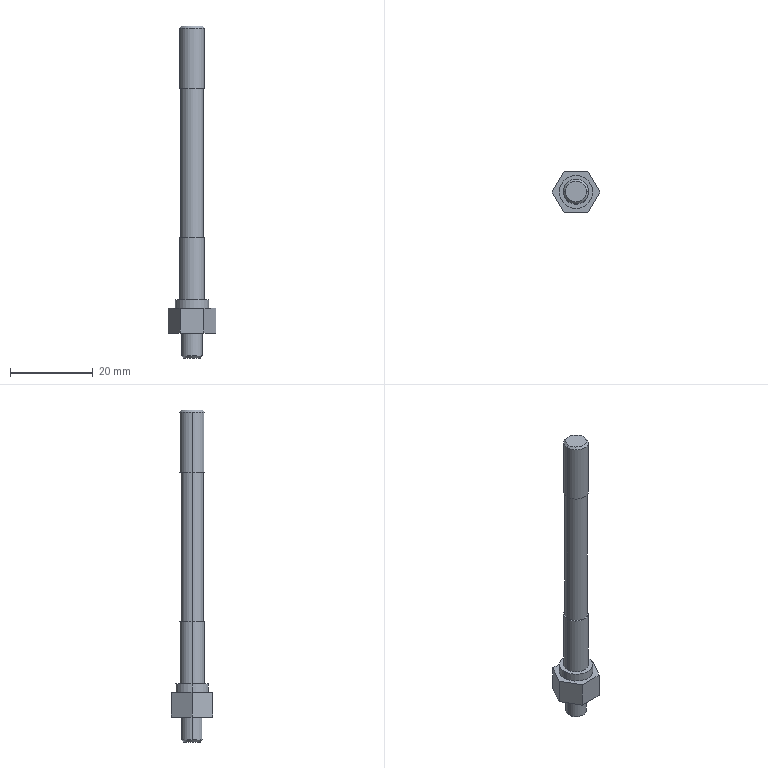Part | SolidWorks | features ICE 3, Chamfer 2, Extrusion 1, RefAxis 1, RevCut 1 | 1 solid | 27 faces | box 11.547 x 10 x 80 mm | volume 2437 mm3 | plane 13 | cylinder 10 | cone 4 | commonest cylinder face diameters 6 x4 5 x2 5.5 x2 8 x2
STEP:
#1=CARTESIAN_POINT('',(-2.,0.,-6.));
#2=VERTEX_POINT('',#1);
#3=CARTESIAN_POINT('',(2.,0.,-6.));
#4=VERTEX_POINT('',#3);
#5=CARTESIAN_POINT('',(0.,0.,-6.));
#6=DIRECTION('',(0.,0.,-1.));
#7=DIRECTION('',(-1.,0.,0.));
#8=AXIS2_PLACEMENT_3D('',#5,#6,#7);
#9=CIRCLE('',#8,2.);
#10=EDGE_CURVE('',#2,#4,#9,.T.);
#11=ORIENTED_EDGE('',*,*,#10,.F.);
#12=CARTESIAN_POINT('',(-2.5,0.,-5.5));
#13=VERTEX_POINT('',#12);
#14=CARTESIAN_POINT('',(-2.,0.,-6.));
#15=DIRECTION('',(-0.7071,0.,0.7071));
#16=VECTOR('',#15,1000.);
#17=LINE('',#14,#16);
#18=EDGE_CURVE('',#2,#13,#17,.T.);
#19=ORIENTED_EDGE('',*,*,#18,.T.);
#20=CARTESIAN_POINT('',(2.5,0.,-5.5));
#21=VERTEX_POINT('',#20);
#22=CARTESIAN_POINT('',(0.,0.,-5.5));
#23=DIRECTION('',(0.,0.,1.));
#24=DIRECTION('',(-1.,0.,0.));
#25=AXIS2_PLACEMENT_3D('',#22,#23,#24);
#26=CIRCLE('',#25,2.5);
#27=EDGE_CURVE('',#21,#13,#26,.T.);
#28=ORIENTED_EDGE('',*,*,#27,.F.);
#29=CARTESIAN_POINT('',(2.,0.,-6.));
#30=DIRECTION('',(0.7071,0.,0.7071));
#31=VECTOR('',#30,1000.);
#32=LINE('',#29,#31);
#33=EDGE_CURVE('',#4,#21,#32,.T.);
#34=ORIENTED_EDGE('',*,*,#33,.F.);
#35=EDGE_LOOP('',(#11,#19,#28,#34));
#36=FACE_OUTER_BOUND('',#35,.T.);
#37=CARTESIAN_POINT('',(0.,0.,-6.));
#38=DIRECTION('',(0.,0.,1.));
#39=DIRECTION('',(1.,0.,0.));
#40=AXIS2_PLACEMENT_3D('',#37,#38,#39);
#41=CONICAL_SURFACE('',#40,2.,0.7854);
#42=ADVANCED_FACE('',(#36),#41,.T.);
#43=CARTESIAN_POINT('',(-3.,0.,73.5));
#44=VERTEX_POINT('',#43);
#45=CARTESIAN_POINT('',(3.,0.,73.5));
#46=VERTEX_POINT('',#45);
#47=CARTESIAN_POINT('',(0.,0.,73.5));
#48=DIRECTION('',(0.,0.,-1.));
#49=DIRECTION('',(1.,0.,0.));
#50=AXIS2_PLACEMENT_3D('',#47,#48,#49);
#51=CIRCLE('',#50,3.);
#52=EDGE_CURVE('',#44,#46,#51,.T.);
#53=ORIENTED_EDGE('',*,*,#52,.T.);
#54=CARTESIAN_POINT('',(3.,0.,59.));
#55=VERTEX_POINT('',#54);
#56=CARTESIAN_POINT('',(3.,0.,74.));
#57=DIRECTION('',(0.,0.,-1.));
#58=VECTOR('',#57,1000.);
#59=LINE('',#56,#58);
#60=EDGE_CURVE('',#46,#55,#59,.T.);
#61=ORIENTED_EDGE('',*,*,#60,.T.);
#62=CARTESIAN_POINT('',(-3.,0.,59.));
#63=VERTEX_POINT('',#62);
#64=CARTESIAN_POINT('',(0.,0.,59.));
#65=DIRECTION('',(0.,0.,1.));
#66=DIRECTION('',(1.,0.,0.));
#67=AXIS2_PLACEMENT_3D('',#64,#65,#66);
#68=CIRCLE('',#67,3.);
#69=EDGE_CURVE('',#55,#63,#68,.T.);
#70=ORIENTED_EDGE('',*,*,#69,.T.);
#71=CARTESIAN_POINT('',(-3.,0.,74.));
#72=DIRECTION('',(0.,0.,-1.));
#73=VECTOR('',#72,1000.);
#74=LINE('',#71,#73);
#75=EDGE_CURVE('',#44,#63,#74,.T.);
#76=ORIENTED_EDGE('',*,*,#75,.F.);
#77=EDGE_LOOP('',(#53,#61,#70,#76));
#78=FACE_OUTER_BOUND('',#77,.T.);
#79=CARTESIAN_POINT('',(0.,0.,74.));
#80=DIRECTION('',(0.,0.,-1.));
#81=DIRECTION('',(-1.,0.,0.));
#82=AXIS2_PLACEMENT_3D('',#79,#80,#81);
#83=CYLINDRICAL_SURFACE('',#82,3.);
#84=ADVANCED_FACE('',(#78),#83,.T.);
#85=CARTESIAN_POINT('',(2.5,0.,74.));
#86=VERTEX_POINT('',#85);
#87=CARTESIAN_POINT('',(-2.5,0.,74.));
#88=VERTEX_POINT('',#87);
#89=CARTESIAN_POINT('',(0.,0.,74.));
#90=DIRECTION('',(0.,0.,1.));
#91=DIRECTION('',(1.,0.,0.));
#92=AXIS2_PLACEMENT_3D('',#89,#90,#91);
#93=CIRCLE('',#92,2.5);
#94=EDGE_CURVE('',#86,#88,#93,.T.);
#95=ORIENTED_EDGE('',*,*,#94,.F.);
#96=CARTESIAN_POINT('',(2.5,0.,74.));
#97=DIRECTION('',(0.7071,0.,-0.7071));
#98=VECTOR('',#97,1000.);
#99=LINE('',#96,#98);
#100=EDGE_CURVE('',#86,#46,#99,.T.);
#101=ORIENTED_EDGE('',*,*,#100,.T.);
#102=ORIENTED_EDGE('',*,*,#52,.F.);
#103=CARTESIAN_POINT('',(-2.5,0.,74.));
#104=DIRECTION('',(-0.7071,0.,-0.7071));
#105=VECTOR('',#104,1000.);
#106=LINE('',#103,#105);
#107=EDGE_CURVE('',#88,#44,#106,.T.);
#108=ORIENTED_EDGE('',*,*,#107,.F.);
#109=EDGE_LOOP('',(#95,#101,#102,#108));
#110=FACE_OUTER_BOUND('',#109,.T.);
#111=CARTESIAN_POINT('',(0.,0.,74.));
#112=DIRECTION('',(0.,0.,-1.));
#113=DIRECTION('',(-1.,0.,0.));
#114=AXIS2_PLACEMENT_3D('',#111,#112,#113);
#115=CONICAL_SURFACE('',#114,2.5,0.7854);
#116=ADVANCED_FACE('',(#110),#115,.T.);
#117=CARTESIAN_POINT('',(2.75,0.,23.));
#118=VERTEX_POINT('',#117);
#119=CARTESIAN_POINT('',(-2.75,0.,23.));
#120=VERTEX_POINT('',#119);
#121=CARTESIAN_POINT('',(0.,0.,23.));
#122=DIRECTION('',(0.,0.,1.));
#123=DIRECTION('',(1.,0.,0.));
#124=AXIS2_PLACEMENT_3D('',#121,#122,#123);
#125=CIRCLE('',#124,2.75);
#126=EDGE_CURVE('',#118,#120,#125,.T.);
#127=ORIENTED_EDGE('',*,*,#126,.T.);
#128=CARTESIAN_POINT('',(-2.75,0.,59.));
#129=VERTEX_POINT('',#128);
#130=CARTESIAN_POINT('',(-2.75,0.,73.5));
#131=DIRECTION('',(0.,0.,1.));
#132=VECTOR('',#131,1000.);
#133=LINE('',#130,#132);
#134=EDGE_CURVE('',#120,#129,#133,.T.);
#135=ORIENTED_EDGE('',*,*,#134,.T.);
#136=CARTESIAN_POINT('',(2.75,0.,59.));
#137=VERTEX_POINT('',#136);
#138=CARTESIAN_POINT('',(0.,0.,59.));
#139=DIRECTION('',(0.,0.,1.));
#140=DIRECTION('',(1.,0.,0.));
#141=AXIS2_PLACEMENT_3D('',#138,#139,#140);
#142=CIRCLE('',#141,2.75);
#143=EDGE_CURVE('',#137,#129,#142,.T.);
#144=ORIENTED_EDGE('',*,*,#143,.F.);
#145=CARTESIAN_POINT('',(2.75,0.,73.5));
#146=DIRECTION('',(0.,0.,1.));
#147=VECTOR('',#146,1000.);
#148=LINE('',#145,#147);
#149=EDGE_CURVE('',#118,#137,#148,.T.);
#150=ORIENTED_EDGE('',*,*,#149,.F.);
#151=EDGE_LOOP('',(#127,#135,#144,#150));
#152=FACE_OUTER_BOUND('',#151,.T.);
#153=CARTESIAN_POINT('',(0.,0.,73.5));
#154=DIRECTION('',(0.,0.,1.));
#155=DIRECTION('',(1.,0.,0.));
#156=AXIS2_PLACEMENT_3D('',#153,#154,#155);
#157=CYLINDRICAL_SURFACE('',#156,2.75);
#158=ADVANCED_FACE('',(#152),#157,.T.);
#159=CARTESIAN_POINT('',(-3.,0.,23.));
#160=VERTEX_POINT('',#159);
#161=CARTESIAN_POINT('',(3.,0.,23.));
#162=VERTEX_POINT('',#161);
#163=CARTESIAN_POINT('',(0.,0.,23.));
#164=DIRECTION('',(0.,0.,-1.));
#165=DIRECTION('',(-1.,0.,0.));
#166=AXIS2_PLACEMENT_3D('',#163,#164,#165);
#167=CIRCLE('',#166,3.);
#168=EDGE_CURVE('',#160,#162,#167,.T.);
#169=ORIENTED_EDGE('',*,*,#168,.T.);
#170=CARTESIAN_POINT('',(3.,0.,8.));
#171=VERTEX_POINT('',#170);
#172=CARTESIAN_POINT('',(3.,0.,74.));
#173=DIRECTION('',(0.,0.,-1.));
#174=VECTOR('',#173,1000.);
#175=LINE('',#172,#174);
#176=EDGE_CURVE('',#162,#171,#175,.T.);
#177=ORIENTED_EDGE('',*,*,#176,.T.);
#178=CARTESIAN_POINT('',(-3.,0.,8.));
#179=VERTEX_POINT('',#178);
#180=CARTESIAN_POINT('',(0.,0.,8.));
#181=DIRECTION('',(0.,0.,1.));
#182=DIRECTION('',(1.,0.,0.));
#183=AXIS2_PLACEMENT_3D('',#180,#181,#182);
#184=CIRCLE('',#183,3.);
#185=EDGE_CURVE('',#171,#179,#184,.T.);
#186=ORIENTED_EDGE('',*,*,#185,.T.);
#187=CARTESIAN_POINT('',(-3.,0.,74.));
#188=DIRECTION('',(0.,0.,-1.));
#189=VECTOR('',#188,1000.);
#190=LINE('',#187,#189);
#191=EDGE_CURVE('',#160,#179,#190,.T.);
#192=ORIENTED_EDGE('',*,*,#191,.F.);
#193=EDGE_LOOP('',(#169,#177,#186,#192));
#194=FACE_OUTER_BOUND('',#193,.T.);
#195=CARTESIAN_POINT('',(0.,0.,74.));
#196=DIRECTION('',(0.,0.,-1.));
#197=DIRECTION('',(-1.,0.,0.));
#198=AXIS2_PLACEMENT_3D('',#195,#196,#197);
#199=CYLINDRICAL_SURFACE('',#198,3.);
#200=ADVANCED_FACE('',(#194),#199,.T.);
#201=CARTESIAN_POINT('',(4.,0.,8.));
#202=VERTEX_POINT('',#201);
#203=CARTESIAN_POINT('',(-4.,0.,8.));
#204=VERTEX_POINT('',#203);
#205=CARTESIAN_POINT('',(0.,0.,8.));
#206=DIRECTION('',(0.,0.,1.));
#207=DIRECTION('',(1.,0.,0.));
#208=AXIS2_PLACEMENT_3D('',#205,#206,#207);
#209=CIRCLE('',#208,4.);
#210=EDGE_CURVE('',#202,#204,#209,.T.);
#211=ORIENTED_EDGE('',*,*,#210,.F.);
#212=CARTESIAN_POINT('',(4.,0.,6.));
#213=VERTEX_POINT('',#212);
#214=CARTESIAN_POINT('',(4.,0.,8.));
#215=DIRECTION('',(0.,0.,-1.));
#216=VECTOR('',#215,1000.);
#217=LINE('',#214,#216);
#218=EDGE_CURVE('',#202,#213,#217,.T.);
#219=ORIENTED_EDGE('',*,*,#218,.T.);
#220=CARTESIAN_POINT('',(-4.,0.,6.));
#221=VERTEX_POINT('',#220);
#222=CARTESIAN_POINT('',(0.,0.,6.));
#223=DIRECTION('',(0.,0.,1.));
#224=DIRECTION('',(1.,0.,0.));
#225=AXIS2_PLACEMENT_3D('',#222,#223,#224);
#226=CIRCLE('',#225,4.);
#227=EDGE_CURVE('',#213,#221,#226,.T.);
#228=ORIENTED_EDGE('',*,*,#227,.T.);
#229=CARTESIAN_POINT('',(-4.,0.,8.));
#230=DIRECTION('',(0.,0.,-1.));
#231=VECTOR('',#230,1000.);
#232=LINE('',#229,#231);
#233=EDGE_CURVE('',#204,#221,#232,.T.);
#234=ORIENTED_EDGE('',*,*,#233,.F.);
#235=EDGE_LOOP('',(#211,#219,#228,#234));
#236=FACE_OUTER_BOUND('',#235,.T.);
#237=CARTESIAN_POINT('',(0.,0.,8.));
#238=DIRECTION('',(0.,0.,-1.));
#239=DIRECTION('',(-1.,0.,0.));
#240=AXIS2_PLACEMENT_3D('',#237,#238,#239);
#241=CYLINDRICAL_SURFACE('',#240,4.);
#242=ADVANCED_FACE('',(#236),#241,.T.);
#243=ORIENTED_EDGE('',*,*,#27,.T.);
#244=CARTESIAN_POINT('',(-2.5,0.,0.));
#245=VERTEX_POINT('',#244);
#246=CARTESIAN_POINT('',(-2.5,0.,-6.));
#247=DIRECTION('',(0.,0.,1.));
#248=VECTOR('',#247,1000.);
#249=LINE('',#246,#248);
#250=EDGE_CURVE('',#13,#245,#249,.T.);
#251=ORIENTED_EDGE('',*,*,#250,.T.);
#252=CARTESIAN_POINT('',(2.5,0.,0.));
#253=VERTEX_POINT('',#252);
#254=CARTESIAN_POINT('',(0.,0.,0.));
#255=DIRECTION('',(0.,0.,-1.));
#256=DIRECTION('',(1.,0.,0.));
#257=AXIS2_PLACEMENT_3D('',#254,#255,#256);
#258=CIRCLE('',#257,2.5);
#259=EDGE_CURVE('',#245,#253,#258,.T.);
#260=ORIENTED_EDGE('',*,*,#259,.T.);
#261=CARTESIAN_POINT('',(2.5,0.,-6.));
#262=DIRECTION('',(0.,0.,1.));
#263=VECTOR('',#262,1000.);
#264=LINE('',#261,#263);
#265=EDGE_CURVE('',#21,#253,#264,.T.);
#266=ORIENTED_EDGE('',*,*,#265,.F.);
#267=EDGE_LOOP('',(#243,#251,#260,#266));
#268=FACE_OUTER_BOUND('',#267,.T.);
#269=CARTESIAN_POINT('',(0.,0.,-6.));
#270=DIRECTION('',(0.,0.,1.));
#271=DIRECTION('',(1.,0.,0.));
#272=AXIS2_PLACEMENT_3D('',#269,#270,#271);
#273=CYLINDRICAL_SURFACE('',#272,2.5);
#274=ADVANCED_FACE('',(#268),#273,.T.);
#275=CARTESIAN_POINT('',(0.,0.,8.));
#276=DIRECTION('',(0.,0.,1.));
#277=DIRECTION('',(1.,0.,0.));
#278=AXIS2_PLACEMENT_3D('',#275,#276,#277);
#279=CIRCLE('',#278,4.);
#280=EDGE_CURVE('',#204,#202,#279,.T.);
#281=ORIENTED_EDGE('',*,*,#280,.T.);
#282=ORIENTED_EDGE('',*,*,#210,.T.);
#283=EDGE_LOOP('',(#281,#282));
#284=FACE_OUTER_BOUND('',#283,.T.);
#285=CARTESIAN_POINT('',(0.,0.,8.));
#286=DIRECTION('',(0.,0.,1.));
#287=DIRECTION('',(1.,0.,0.));
#288=AXIS2_PLACEMENT_3D('',#285,#286,#287);
#289=CIRCLE('',#288,3.);
#290=EDGE_CURVE('',#179,#171,#289,.T.);
#291=ORIENTED_EDGE('',*,*,#290,.F.);
#292=ORIENTED_EDGE('',*,*,#185,.F.);
#293=EDGE_LOOP('',(#291,#292));
#294=FACE_BOUND('',#293,.T.);
#295=CARTESIAN_POINT('',(0.,0.,8.));
#296=DIRECTION('',(0.,0.,1.));
#297=DIRECTION('',(1.,0.,0.));
#298=AXIS2_PLACEMENT_3D('',#295,#296,#297);
#299=PLANE('',#298);
#300=ADVANCED_FACE('',(#284,#294),#299,.T.);
#301=CARTESIAN_POINT('',(2.887,-5.,6.));
#302=VERTEX_POINT('',#301);
#303=CARTESIAN_POINT('',(5.774,0.,6.));
#304=VERTEX_POINT('',#303);
#305=CARTESIAN_POINT('',(2.887,-5.,6.));
#306=DIRECTION('',(0.5,0.866,0.));
#307=VECTOR('',#306,1000.);
#308=LINE('',#305,#307);
#309=EDGE_CURVE('',#302,#304,#308,.T.);
#310=ORIENTED_EDGE('',*,*,#309,.T.);
#311=CARTESIAN_POINT('',(2.887,5.,6.));
#312=VERTEX_POINT('',#311);
#313=CARTESIAN_POINT('',(5.774,0.,6.));
#314=DIRECTION('',(-0.5,0.866,0.));
#315=VECTOR('',#314,1000.);
#316=LINE('',#313,#315);
#317=EDGE_CURVE('',#304,#312,#316,.T.);
#318=ORIENTED_EDGE('',*,*,#317,.T.);
#319=CARTESIAN_POINT('',(-2.887,5.,6.));
#320=VERTEX_POINT('',#319);
#321=CARTESIAN_POINT('',(2.887,5.,6.));
#322=DIRECTION('',(-1.,0.,0.));
#323=VECTOR('',#322,1000.);
#324=LINE('',#321,#323);
#325=EDGE_CURVE('',#312,#320,#324,.T.);
#326=ORIENTED_EDGE('',*,*,#325,.T.);
#327=CARTESIAN_POINT('',(-5.774,0.,6.));
#328=VERTEX_POINT('',#327);
#329=CARTESIAN_POINT('',(-2.887,5.,6.));
#330=DIRECTION('',(-0.5,-0.866,0.));
#331=VECTOR('',#330,1000.);
#332=LINE('',#329,#331);
#333=EDGE_CURVE('',#320,#328,#332,.T.);
#334=ORIENTED_EDGE('',*,*,#333,.T.);
#335=CARTESIAN_POINT('',(-2.887,-5.,6.));
#336=VERTEX_POINT('',#335);
#337=CARTESIAN_POINT('',(-5.774,0.,6.));
#338=DIRECTION('',(0.5,-0.866,0.));
#339=VECTOR('',#338,1000.);
#340=LINE('',#337,#339);
#341=EDGE_CURVE('',#328,#336,#340,.T.);
#342=ORIENTED_EDGE('',*,*,#341,.T.);
#343=CARTESIAN_POINT('',(-2.887,-5.,6.));
#344=DIRECTION('',(1.,0.,0.));
#345=VECTOR('',#344,1000.);
#346=LINE('',#343,#345);
#347=EDGE_CURVE('',#336,#302,#346,.T.);
#348=ORIENTED_EDGE('',*,*,#347,.T.);
#349=EDGE_LOOP('',(#310,#318,#326,#334,#342,#348));
#350=FACE_OUTER_BOUND('',#349,.T.);
#351=CARTESIAN_POINT('',(0.,0.,6.));
#352=DIRECTION('',(0.,0.,1.));
#353=DIRECTION('',(1.,0.,0.));
#354=AXIS2_PLACEMENT_3D('',#351,#352,#353);
#355=CIRCLE('',#354,4.);
#356=EDGE_CURVE('',#221,#213,#355,.T.);
#357=ORIENTED_EDGE('',*,*,#356,.F.);
#358=ORIENTED_EDGE('',*,*,#227,.F.);
#359=EDGE_LOOP('',(#357,#358));
#360=FACE_BOUND('',#359,.T.);
#361=CARTESIAN_POINT('',(5.774,0.,6.));
#362=DIRECTION('',(0.,0.,1.));
#363=DIRECTION('',(1.,0.,0.));
#364=AXIS2_PLACEMENT_3D('',#361,#362,#363);
#365=PLANE('',#364);
#366=ADVANCED_FACE('',(#350,#360),#365,.T.);
#367=CARTESIAN_POINT('',(2.887,-5.,0.));
#368=VERTEX_POINT('',#367);
#369=CARTESIAN_POINT('',(5.774,0.,0.));
#370=VERTEX_POINT('',#369);
#371=CARTESIAN_POINT('',(2.887,-5.,0.));
#372=DIRECTION('',(0.5,0.866,0.));
#373=VECTOR('',#372,1000.);
#374=LINE('',#371,#373);
#375=EDGE_CURVE('',#368,#370,#374,.T.);
#376=ORIENTED_EDGE('',*,*,#375,.F.);
#377=CARTESIAN_POINT('',(-2.887,-5.,0.));
#378=VERTEX_POINT('',#377);
#379=CARTESIAN_POINT('',(-2.887,-5.,0.));
#380=DIRECTION('',(1.,0.,0.));
#381=VECTOR('',#380,1000.);
#382=LINE('',#379,#381);
#383=EDGE_CURVE('',#378,#368,#382,.T.);
#384=ORIENTED_EDGE('',*,*,#383,.F.);
#385=CARTESIAN_POINT('',(-5.774,0.,0.));
#386=VERTEX_POINT('',#385);
#387=CARTESIAN_POINT('',(-5.774,0.,0.));
#388=DIRECTION('',(0.5,-0.866,0.));
#389=VECTOR('',#388,1000.);
#390=LINE('',#387,#389);
#391=EDGE_CURVE('',#386,#378,#390,.T.);
#392=ORIENTED_EDGE('',*,*,#391,.F.);
#393=CARTESIAN_POINT('',(-2.887,5.,0.));
#394=VERTEX_POINT('',#393);
#395=CARTESIAN_POINT('',(-2.887,5.,0.));
#396=DIRECTION('',(-0.5,-0.866,0.));
#397=VECTOR('',#396,1000.);
#398=LINE('',#395,#397);
#399=EDGE_CURVE('',#394,#386,#398,.T.);
#400=ORIENTED_EDGE('',*,*,#399,.F.);
#401=CARTESIAN_POINT('',(2.887,5.,0.));
#402=VERTEX_POINT('',#401);
#403=CARTESIAN_POINT('',(2.887,5.,0.));
#404=DIRECTION('',(-1.,0.,0.));
#405=VECTOR('',#404,1000.);
#406=LINE('',#403,#405);
#407=EDGE_CURVE('',#402,#394,#406,.T.);
#408=ORIENTED_EDGE('',*,*,#407,.F.);
#409=CARTESIAN_POINT('',(5.774,0.,0.));
#410=DIRECTION('',(-0.5,0.866,0.));
#411=VECTOR('',#410,1000.);
#412=LINE('',#409,#411);
#413=EDGE_CURVE('',#370,#402,#412,.T.);
#414=ORIENTED_EDGE('',*,*,#413,.F.);
#415=EDGE_LOOP('',(#376,#384,#392,#400,#408,#414));
#416=FACE_OUTER_BOUND('',#415,.T.);
#417=CARTESIAN_POINT('',(0.,0.,0.));
#418=DIRECTION('',(0.,0.,-1.));
#419=DIRECTION('',(1.,0.,0.));
#420=AXIS2_PLACEMENT_3D('',#417,#418,#419);
#421=CIRCLE('',#420,2.5);
#422=EDGE_CURVE('',#253,#245,#421,.T.);
#423=ORIENTED_EDGE('',*,*,#422,.F.);
#424=ORIENTED_EDGE('',*,*,#259,.F.);
#425=EDGE_LOOP('',(#423,#424));
#426=FACE_BOUND('',#425,.T.);
#427=CARTESIAN_POINT('',(5.774,0.,0.));
#428=DIRECTION('',(0.,0.,1.));
#429=DIRECTION('',(1.,0.,0.));
#430=AXIS2_PLACEMENT_3D('',#427,#428,#429);
#431=PLANE('',#430);
#432=ADVANCED_FACE('',(#416,#426),#431,.F.);
#433=ORIENTED_EDGE('',*,*,#375,.T.);
#434=CARTESIAN_POINT('',(5.774,0.,6.));
#435=DIRECTION('',(0.,0.,-1.));
#436=VECTOR('',#435,1000.);
#437=LINE('',#434,#436);
#438=EDGE_CURVE('',#304,#370,#437,.T.);
#439=ORIENTED_EDGE('',*,*,#438,.F.);
#440=ORIENTED_EDGE('',*,*,#309,.F.);
#441=CARTESIAN_POINT('',(2.887,-5.,6.));
#442=DIRECTION('',(0.,0.,-1.));
#443=VECTOR('',#442,1000.);
#444=LINE('',#441,#443);
#445=EDGE_CURVE('',#302,#368,#444,.T.);
#446=ORIENTED_EDGE('',*,*,#445,.T.);
#447=EDGE_LOOP('',(#433,#439,#440,#446));
#448=FACE_OUTER_BOUND('',#447,.T.);
#449=CARTESIAN_POINT('',(2.887,-5.,6.));
#450=DIRECTION('',(-0.866,0.5,0.));
#451=DIRECTION('',(-0.5,-0.866,0.));
#452=AXIS2_PLACEMENT_3D('',#449,#450,#451);
#453=PLANE('',#452);
#454=ADVANCED_FACE('',(#448),#453,.F.);
#455=ORIENTED_EDGE('',*,*,#413,.T.);
#456=CARTESIAN_POINT('',(2.887,5.,6.));
#457=DIRECTION('',(0.,0.,-1.));
#458=VECTOR('',#457,1000.);
#459=LINE('',#456,#458);
#460=EDGE_CURVE('',#312,#402,#459,.T.);
#461=ORIENTED_EDGE('',*,*,#460,.F.);
#462=ORIENTED_EDGE('',*,*,#317,.F.);
#463=ORIENTED_EDGE('',*,*,#438,.T.);
#464=EDGE_LOOP('',(#455,#461,#462,#463));
#465=FACE_OUTER_BOUND('',#464,.T.);
#466=CARTESIAN_POINT('',(5.774,0.,6.));
#467=DIRECTION('',(-0.866,-0.5,0.));
#468=DIRECTION('',(0.5,-0.866,0.));
#469=AXIS2_PLACEMENT_3D('',#466,#467,#468);
#470=PLANE('',#469);
#471=ADVANCED_FACE('',(#465),#470,.F.);
#472=ORIENTED_EDGE('',*,*,#407,.T.);
#473=CARTESIAN_POINT('',(-2.887,5.,6.));
#474=DIRECTION('',(0.,0.,-1.));
#475=VECTOR('',#474,1000.);
#476=LINE('',#473,#475);
#477=EDGE_CURVE('',#320,#394,#476,.T.);
#478=ORIENTED_EDGE('',*,*,#477,.F.);
#479=ORIENTED_EDGE('',*,*,#325,.F.);
#480=ORIENTED_EDGE('',*,*,#460,.T.);
#481=EDGE_LOOP('',(#472,#478,#479,#480));
#482=FACE_OUTER_BOUND('',#481,.T.);
#483=CARTESIAN_POINT('',(2.887,5.,6.));
#484=DIRECTION('',(0.,-1.,0.));
#485=DIRECTION('',(0.,0.,-1.));
#486=AXIS2_PLACEMENT_3D('',#483,#484,#485);
#487=PLANE('',#486);
#488=ADVANCED_FACE('',(#482),#487,.F.);
#489=ORIENTED_EDGE('',*,*,#399,.T.);
#490=CARTESIAN_POINT('',(-5.774,0.,6.));
#491=DIRECTION('',(0.,0.,-1.));
#492=VECTOR('',#491,1000.);
#493=LINE('',#490,#492);
#494=EDGE_CURVE('',#328,#386,#493,.T.);
#495=ORIENTED_EDGE('',*,*,#494,.F.);
#496=ORIENTED_EDGE('',*,*,#333,.F.);
#497=ORIENTED_EDGE('',*,*,#477,.T.);
#498=EDGE_LOOP('',(#489,#495,#496,#497));
#499=FACE_OUTER_BOUND('',#498,.T.);
#500=CARTESIAN_POINT('',(-2.887,5.,6.));
#501=DIRECTION('',(0.866,-0.5,0.));
#502=DIRECTION('',(0.5,0.866,0.));
#503=AXIS2_PLACEMENT_3D('',#500,#501,#502);
#504=PLANE('',#503);
#505=ADVANCED_FACE('',(#499),#504,.F.);
#506=ORIENTED_EDGE('',*,*,#391,.T.);
#507=CARTESIAN_POINT('',(-2.887,-5.,6.));
#508=DIRECTION('',(0.,0.,-1.));
#509=VECTOR('',#508,1000.);
#510=LINE('',#507,#509);
#511=EDGE_CURVE('',#336,#378,#510,.T.);
#512=ORIENTED_EDGE('',*,*,#511,.F.);
#513=ORIENTED_EDGE('',*,*,#341,.F.);
#514=ORIENTED_EDGE('',*,*,#494,.T.);
#515=EDGE_LOOP('',(#506,#512,#513,#514));
#516=FACE_OUTER_BOUND('',#515,.T.);
#517=CARTESIAN_POINT('',(-5.774,0.,6.));
#518=DIRECTION('',(0.866,0.5,0.));
#519=DIRECTION('',(-0.5,0.866,0.));
#520=AXIS2_PLACEMENT_3D('',#517,#518,#519);
#521=PLANE('',#520);
#522=ADVANCED_FACE('',(#516),#521,.F.);
#523=ORIENTED_EDGE('',*,*,#383,.T.);
#524=ORIENTED_EDGE('',*,*,#445,.F.);
#525=ORIENTED_EDGE('',*,*,#347,.F.);
#526=ORIENTED_EDGE('',*,*,#511,.T.);
#527=EDGE_LOOP('',(#523,#524,#525,#526));
#528=FACE_OUTER_BOUND('',#527,.T.);
#529=CARTESIAN_POINT('',(-2.887,-5.,6.));
#530=DIRECTION('',(0.,1.,0.));
#531=DIRECTION('',(-1.,0.,0.));
#532=AXIS2_PLACEMENT_3D('',#529,#530,#531);
#533=PLANE('',#532);
#534=ADVANCED_FACE('',(#528),#533,.F.);
#535=ORIENTED_EDGE('',*,*,#250,.F.);
#536=CARTESIAN_POINT('',(0.,0.,-5.5));
#537=DIRECTION('',(0.,0.,1.));
#538=DIRECTION('',(-1.,0.,0.));
#539=AXIS2_PLACEMENT_3D('',#536,#537,#538);
#540=CIRCLE('',#539,2.5);
#541=EDGE_CURVE('',#13,#21,#540,.T.);
#542=ORIENTED_EDGE('',*,*,#541,.T.);
#543=ORIENTED_EDGE('',*,*,#265,.T.);
#544=ORIENTED_EDGE('',*,*,#422,.T.);
#545=EDGE_LOOP('',(#535,#542,#543,#544));
#546=FACE_OUTER_BOUND('',#545,.T.);
#547=CARTESIAN_POINT('',(0.,0.,-6.));
#548=DIRECTION('',(0.,0.,1.));
#549=DIRECTION('',(1.,0.,0.));
#550=AXIS2_PLACEMENT_3D('',#547,#548,#549);
#551=CYLINDRICAL_SURFACE('',#550,2.5);
#552=ADVANCED_FACE('',(#546),#551,.T.);
#553=CARTESIAN_POINT('',(0.,0.,-6.));
#554=DIRECTION('',(0.,0.,-1.));
#555=DIRECTION('',(-1.,0.,0.));
#556=AXIS2_PLACEMENT_3D('',#553,#554,#555);
#557=CIRCLE('',#556,2.);
#558=EDGE_CURVE('',#4,#2,#557,.T.);
#559=ORIENTED_EDGE('',*,*,#558,.T.);
#560=ORIENTED_EDGE('',*,*,#10,.T.);
#561=EDGE_LOOP('',(#559,#560));
#562=FACE_OUTER_BOUND('',#561,.T.);
#563=CARTESIAN_POINT('',(0.,0.,-6.));
#564=DIRECTION('',(0.,0.,-1.));
#565=DIRECTION('',(-1.,0.,0.));
#566=AXIS2_PLACEMENT_3D('',#563,#564,#565);
#567=PLANE('',#566);
#568=ADVANCED_FACE('',(#562),#567,.T.);
#569=ORIENTED_EDGE('',*,*,#218,.F.);
#570=ORIENTED_EDGE('',*,*,#280,.F.);
#571=ORIENTED_EDGE('',*,*,#233,.T.);
#572=ORIENTED_EDGE('',*,*,#356,.T.);
#573=EDGE_LOOP('',(#569,#570,#571,#572));
#574=FACE_OUTER_BOUND('',#573,.T.);
#575=CARTESIAN_POINT('',(0.,0.,8.));
#576=DIRECTION('',(0.,0.,-1.));
#577=DIRECTION('',(-1.,0.,0.));
#578=AXIS2_PLACEMENT_3D('',#575,#576,#577);
#579=CYLINDRICAL_SURFACE('',#578,4.);
#580=ADVANCED_FACE('',(#574),#579,.T.);
#581=ORIENTED_EDGE('',*,*,#176,.F.);
#582=CARTESIAN_POINT('',(0.,0.,23.));
#583=DIRECTION('',(0.,0.,-1.));
#584=DIRECTION('',(-1.,0.,0.));
#585=AXIS2_PLACEMENT_3D('',#582,#583,#584);
#586=CIRCLE('',#585,3.);
#587=EDGE_CURVE('',#162,#160,#586,.T.);
#588=ORIENTED_EDGE('',*,*,#587,.T.);
#589=ORIENTED_EDGE('',*,*,#191,.T.);
#590=ORIENTED_EDGE('',*,*,#290,.T.);
#591=EDGE_LOOP('',(#581,#588,#589,#590));
#592=FACE_OUTER_BOUND('',#591,.T.);
#593=CARTESIAN_POINT('',(0.,0.,74.));
#594=DIRECTION('',(0.,0.,-1.));
#595=DIRECTION('',(-1.,0.,0.));
#596=AXIS2_PLACEMENT_3D('',#593,#594,#595);
#597=CYLINDRICAL_SURFACE('',#596,3.);
#598=ADVANCED_FACE('',(#592),#597,.T.);
#599=ORIENTED_EDGE('',*,*,#143,.T.);
#600=CARTESIAN_POINT('',(0.,0.,59.));
#601=DIRECTION('',(0.,0.,1.));
#602=DIRECTION('',(1.,0.,0.));
#603=AXIS2_PLACEMENT_3D('',#600,#601,#602);
#604=CIRCLE('',#603,2.75);
#605=EDGE_CURVE('',#129,#137,#604,.T.);
#606=ORIENTED_EDGE('',*,*,#605,.T.);
#607=EDGE_LOOP('',(#599,#606));
#608=FACE_BOUND('',#607,.T.);
#609=CARTESIAN_POINT('',(0.,0.,59.));
#610=DIRECTION('',(0.,0.,1.));
#611=DIRECTION('',(1.,0.,0.));
#612=AXIS2_PLACEMENT_3D('',#609,#610,#611);
#613=CIRCLE('',#612,3.);
#614=EDGE_CURVE('',#63,#55,#613,.T.);
#615=ORIENTED_EDGE('',*,*,#614,.F.);
#616=ORIENTED_EDGE('',*,*,#69,.F.);
#617=EDGE_LOOP('',(#615,#616));
#618=FACE_OUTER_BOUND('',#617,.T.);
#619=CARTESIAN_POINT('',(2.75,0.,59.));
#620=DIRECTION('',(0.,0.,1.));
#621=DIRECTION('',(1.,0.,0.));
#622=AXIS2_PLACEMENT_3D('',#619,#620,#621);
#623=PLANE('',#622);
#624=ADVANCED_FACE('',(#608,#618),#623,.F.);
#625=ORIENTED_EDGE('',*,*,#126,.F.);
#626=CARTESIAN_POINT('',(0.,0.,23.));
#627=DIRECTION('',(0.,0.,1.));
#628=DIRECTION('',(1.,0.,0.));
#629=AXIS2_PLACEMENT_3D('',#626,#627,#628);
#630=CIRCLE('',#629,2.75);
#631=EDGE_CURVE('',#120,#118,#630,.T.);
#632=ORIENTED_EDGE('',*,*,#631,.F.);
#633=EDGE_LOOP('',(#625,#632));
#634=FACE_BOUND('',#633,.T.);
#635=ORIENTED_EDGE('',*,*,#168,.F.);
#636=ORIENTED_EDGE('',*,*,#587,.F.);
#637=EDGE_LOOP('',(#635,#636));
#638=FACE_OUTER_BOUND('',#637,.T.);
#639=CARTESIAN_POINT('',(2.75,0.,23.));
#640=DIRECTION('',(0.,0.,-1.));
#641=DIRECTION('',(-1.,0.,0.));
#642=AXIS2_PLACEMENT_3D('',#639,#640,#641);
#643=PLANE('',#642);
#644=ADVANCED_FACE('',(#634,#638),#643,.F.);
#645=ORIENTED_EDGE('',*,*,#134,.F.);
#646=ORIENTED_EDGE('',*,*,#631,.T.);
#647=ORIENTED_EDGE('',*,*,#149,.T.);
#648=ORIENTED_EDGE('',*,*,#605,.F.);
#649=EDGE_LOOP('',(#645,#646,#647,#648));
#650=FACE_OUTER_BOUND('',#649,.T.);
#651=CARTESIAN_POINT('',(0.,0.,73.5));
#652=DIRECTION('',(0.,0.,1.));
#653=DIRECTION('',(1.,0.,0.));
#654=AXIS2_PLACEMENT_3D('',#651,#652,#653);
#655=CYLINDRICAL_SURFACE('',#654,2.75);
#656=ADVANCED_FACE('',(#650),#655,.T.);
#657=CARTESIAN_POINT('',(0.,0.,74.));
#658=DIRECTION('',(0.,0.,1.));
#659=DIRECTION('',(1.,0.,0.));
#660=AXIS2_PLACEMENT_3D('',#657,#658,#659);
#661=CIRCLE('',#660,2.5);
#662=EDGE_CURVE('',#88,#86,#661,.T.);
#663=ORIENTED_EDGE('',*,*,#662,.T.);
#664=ORIENTED_EDGE('',*,*,#94,.T.);
#665=EDGE_LOOP('',(#663,#664));
#666=FACE_OUTER_BOUND('',#665,.T.);
#667=CARTESIAN_POINT('',(0.,0.,74.));
#668=DIRECTION('',(0.,0.,1.));
#669=DIRECTION('',(1.,0.,0.));
#670=AXIS2_PLACEMENT_3D('',#667,#668,#669);
#671=PLANE('',#670);
#672=ADVANCED_FACE('',(#666),#671,.T.);
#673=ORIENTED_EDGE('',*,*,#100,.F.);
#674=ORIENTED_EDGE('',*,*,#662,.F.);
#675=ORIENTED_EDGE('',*,*,#107,.T.);
#676=CARTESIAN_POINT('',(0.,0.,73.5));
#677=DIRECTION('',(0.,0.,-1.));
#678=DIRECTION('',(1.,0.,0.));
#679=AXIS2_PLACEMENT_3D('',#676,#677,#678);
#680=CIRCLE('',#679,3.);
#681=EDGE_CURVE('',#46,#44,#680,.T.);
#682=ORIENTED_EDGE('',*,*,#681,.F.);
#683=EDGE_LOOP('',(#673,#674,#675,#682));
#684=FACE_OUTER_BOUND('',#683,.T.);
#685=CARTESIAN_POINT('',(0.,0.,74.));
#686=DIRECTION('',(0.,0.,-1.));
#687=DIRECTION('',(-1.,0.,0.));
#688=AXIS2_PLACEMENT_3D('',#685,#686,#687);
#689=CONICAL_SURFACE('',#688,2.5,0.7854);
#690=ADVANCED_FACE('',(#684),#689,.T.);
#691=ORIENTED_EDGE('',*,*,#60,.F.);
#692=ORIENTED_EDGE('',*,*,#681,.T.);
#693=ORIENTED_EDGE('',*,*,#75,.T.);
#694=ORIENTED_EDGE('',*,*,#614,.T.);
#695=EDGE_LOOP('',(#691,#692,#693,#694));
#696=FACE_OUTER_BOUND('',#695,.T.);
#697=CARTESIAN_POINT('',(0.,0.,74.));
#698=DIRECTION('',(0.,0.,-1.));
#699=DIRECTION('',(-1.,0.,0.));
#700=AXIS2_PLACEMENT_3D('',#697,#698,#699);
#701=CYLINDRICAL_SURFACE('',#700,3.);
#702=ADVANCED_FACE('',(#696),#701,.T.);
#703=ORIENTED_EDGE('',*,*,#18,.F.);
#704=ORIENTED_EDGE('',*,*,#558,.F.);
#705=ORIENTED_EDGE('',*,*,#33,.T.);
#706=ORIENTED_EDGE('',*,*,#541,.F.);
#707=EDGE_LOOP('',(#703,#704,#705,#706));
#708=FACE_OUTER_BOUND('',#707,.T.);
#709=CARTESIAN_POINT('',(0.,0.,-6.));
#710=DIRECTION('',(0.,0.,1.));
#711=DIRECTION('',(1.,0.,0.));
#712=AXIS2_PLACEMENT_3D('',#709,#710,#711);
#713=CONICAL_SURFACE('',#712,2.,0.7854);
#714=ADVANCED_FACE('',(#708),#713,.T.);
#715=CLOSED_SHELL('',(#42,#84,#116,#158,#200,#242,#274,#300,#366,#432,#454,#471,#488,#505,#522,#534,#552,#568,#580,#598,#624,#644,#656,#672,#690,#702,#714));
#716=MANIFOLD_SOLID_BREP('',#715);
#717=CARTESIAN_POINT('',(0.,0.,0.));
#718=DIRECTION('',(0.,0.,1.));
#719=DIRECTION('',(1.,0.,0.));
#720=AXIS2_PLACEMENT_3D('',#717,#718,#719);
#721=(LENGTH_UNIT()NAMED_UNIT(*)SI_UNIT(.MILLI.,.METRE.));
#722=UNCERTAINTY_MEASURE_WITH_UNIT(LENGTH_MEASURE(0.00001),#721,'','');
#723=(NAMED_UNIT(*)PLANE_ANGLE_UNIT()SI_UNIT($,.RADIAN.));
#724=(NAMED_UNIT(*)SI_UNIT($,.STERADIAN.)SOLID_ANGLE_UNIT());
#725=(GEOMETRIC_REPRESENTATION_CONTEXT(3)GLOBAL_UNCERTAINTY_ASSIGNED_CONTEXT((#722))GLOBAL_UNIT_ASSIGNED_CONTEXT((#721,#723,#724))REPRESENTATION_CONTEXT('',''));
#726=ADVANCED_BREP_SHAPE_REPRESENTATION('',(#716,#720),#725);